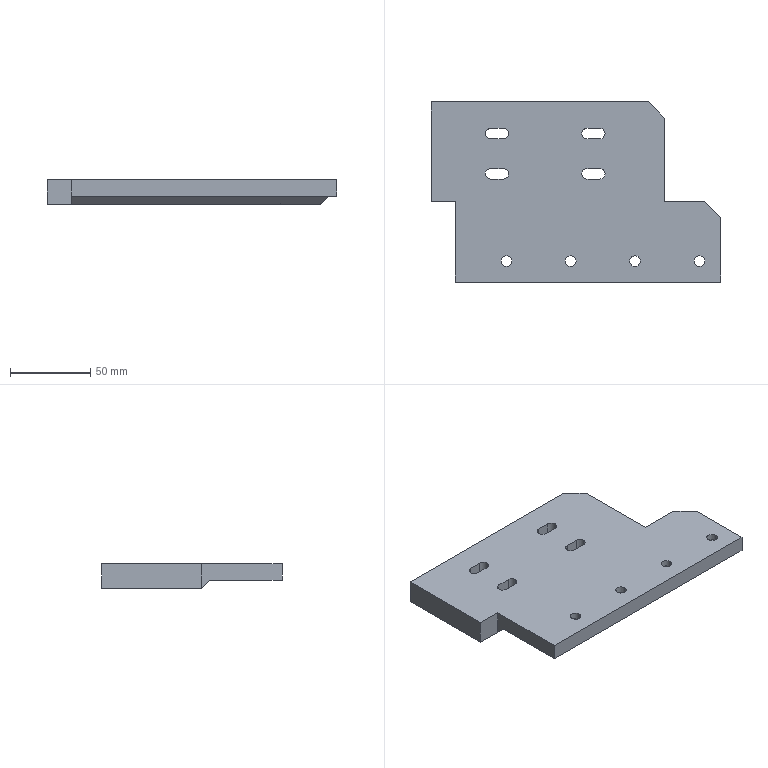Part | STEP file | secondary slingshot input track spacer block | 1 solid | 54 faces | box 180 x 112 x 15 mm | volume 210119 mm3 | cylinder 28 | plane 26 | commonest cylinder face diameters 6.5 x12 6.6 x8 11 x8